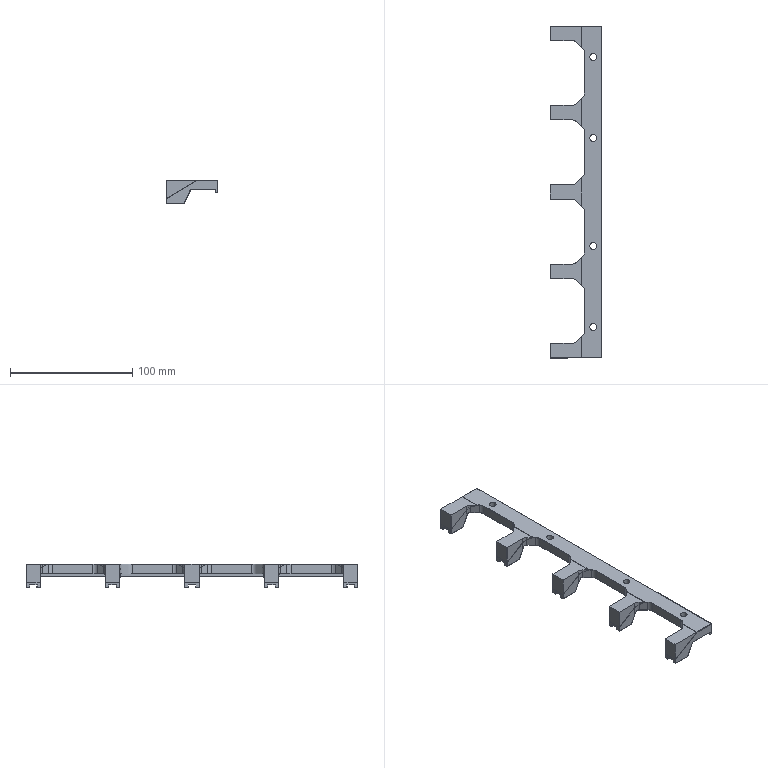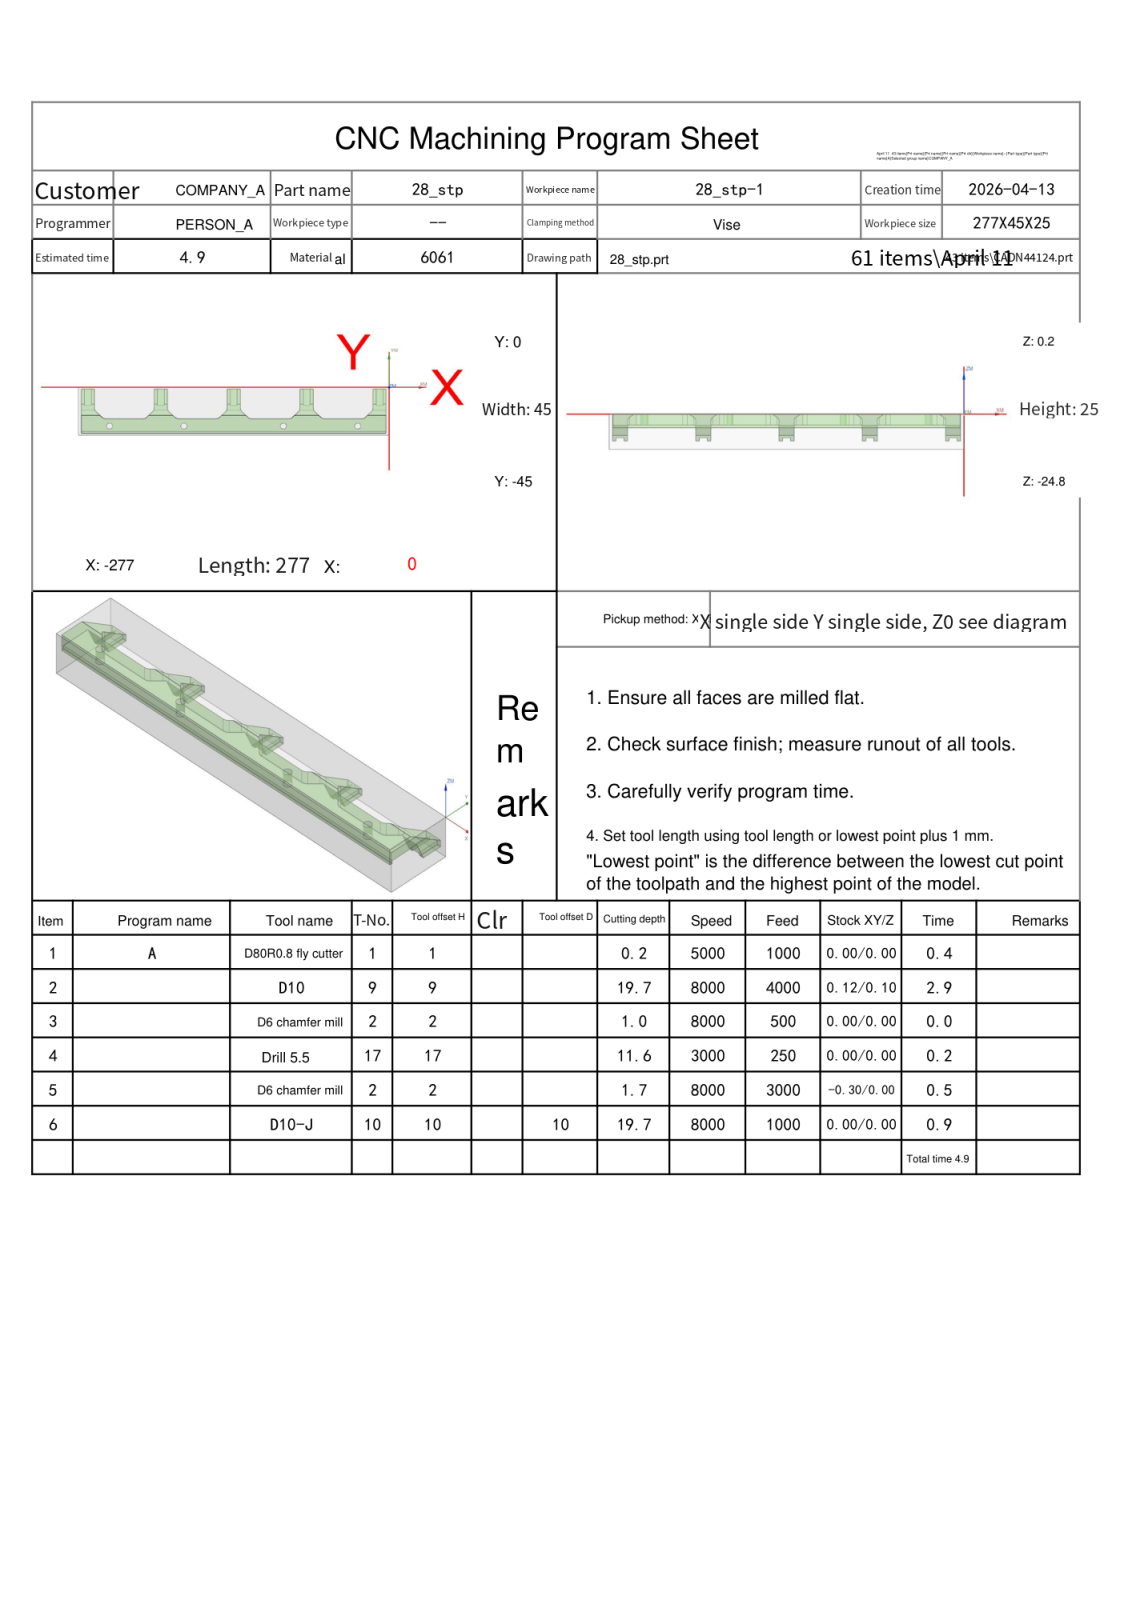NC program | NX | posted by the shop | part box 42 x 271.8 x 19 mm
Lines 2488 to 2830 of 2830:
N3 T02 M06
(D6 chamfer mill  D=6. R=0. H=02 ce=0.00 di=0.10)
G00 G90 G54 X-27.9 Y-36.5 M03 S8000
G43 H02 Z20.
M08
G98 G81 X-27.9 Y-36.5 Z-.8 R1. F500.
X-94.2
X-182.8
X-249.1
G80
G00 Z20.
G91 G28 Z0.0
M05
M09
G91 G28 Z0.0
M01
N4 T17 M06
(drill 5.5 D=5.5 DR_a=118 H=17)
G00 G90 G54 X-27.9 Y-36.5 M03 S3000
G43 H17 Z20.
M08
G98 G83 X-27.9 Y-36.5 Z-11.402 R1. F250. Q3.
X-94.2
X-182.8
X-249.1
G80
G00 Z20.
G91 G28 Z0.0
M05
M09
G91 G28 Z0.0
M01
N5 T02 M06
(D6 chamfer mill  D=6. R=0. H=02 ce=0.00 di=0.00)
G00 G90 G54 X-138.25 Y-45.628 M03 S8000
G43 H02 Z20.
M08
Z2.099
G01 Z-1.499 F3000.
G03 X-138.17 Y-45.328 I-.52 J.3
X-138.47 Y-44.808 I-.6 J0.0
G01 X-138.5 Y-44.8
X-273.9
X-274.154 Y-44.775
X-274.397 Y-44.701
X-274.622 Y-44.581
X-274.819 Y-44.419
X-275.319 Y-43.919
X-275.481 Y-43.722
X-275.601 Y-43.497
X-275.675 Y-43.254
X-275.7 Y-43.
Y-1.7
X-275.675 Y-1.446
X-275.601 Y-1.203
X-275.481 Y-.978
X-275.319 Y-.781
X-275.119 Y-.581
X-274.922 Y-.419
X-274.697 Y-.299
X-274.454 Y-.225
X-274.2 Y-.2
X-262.7
X-262.446 Y-.225
X-262.203 Y-.299
X-261.978 Y-.419
X-261.781 Y-.581
X-261.581 Y-.781
X-261.419 Y-.978
X-261.299 Y-1.203
X-261.225 Y-1.446
X-261.2 Y-1.7
Y-19.429
G03 X-260.116 Y-22.045 I3.7 J0.0
G01 X-255.045 Y-27.116
G03 X-252.429 Y-28.2 I2.616 J2.616
G01 X-219.571
G03 X-216.955 Y-27.116 I0.0 J3.7
G01 X-211.884 Y-22.045
G03 X-210.8 Y-19.429 I-2.616 J2.616
G01 Y-1.7
X-210.775 Y-1.446
X-210.701 Y-1.203
X-210.581 Y-.978
X-210.419 Y-.781
X-210.219 Y-.581
X-210.022 Y-.419
X-209.797 Y-.299
X-209.554 Y-.225
X-209.3 Y-.2
X-197.7
X-197.446 Y-.225
X-197.203 Y-.299
X-196.978 Y-.419
X-196.781 Y-.581
X-196.581 Y-.781
X-196.419 Y-.978
X-196.299 Y-1.203
X-196.225 Y-1.446
X-196.2 Y-1.7
Y-19.429
G03 X-195.116 Y-22.045 I3.7 J0.0
G01 X-190.045 Y-27.116
G03 X-187.429 Y-28.2 I2.616 J2.616
G01 X-154.571
G03 X-151.955 Y-27.116 I0.0 J3.7
G01 X-146.884 Y-22.045
G03 X-145.8 Y-19.429 I-2.616 J2.616
G01 Y-1.7
X-145.775 Y-1.446
X-145.701 Y-1.203
X-145.581 Y-.978
X-145.419 Y-.781
X-145.219 Y-.581
X-145.022 Y-.419
X-144.797 Y-.299
X-144.554 Y-.225
X-144.3 Y-.2
X-132.7
X-132.446 Y-.225
X-132.203 Y-.299
X-131.978 Y-.419
X-131.781 Y-.581
X-131.581 Y-.781
X-131.419 Y-.978
X-131.299 Y-1.203
X-131.225 Y-1.446
X-131.2 Y-1.7
Y-19.429
G03 X-130.116 Y-22.045 I3.7 J0.0
G01 X-125.045 Y-27.116
G03 X-122.429 Y-28.2 I2.616 J2.616
G01 X-89.571
G03 X-86.955 Y-27.116 I0.0 J3.7
G01 X-81.884 Y-22.045
G03 X-80.8 Y-19.429 I-2.616 J2.616
G01 Y-1.7
X-80.775 Y-1.446
X-80.701 Y-1.203
X-80.581 Y-.978
X-80.419 Y-.781
X-80.219 Y-.581
X-80.022 Y-.419
X-79.797 Y-.299
X-79.554 Y-.225
X-79.3 Y-.2
X-67.7
X-67.446 Y-.225
X-67.203 Y-.299
X-66.978 Y-.419
X-66.781 Y-.581
X-66.581 Y-.781
X-66.419 Y-.978
X-66.299 Y-1.203
X-66.225 Y-1.446
X-66.2 Y-1.7
Y-19.429
G03 X-65.116 Y-22.045 I3.7 J0.0
G01 X-60.045 Y-27.116
G03 X-57.429 Y-28.2 I2.616 J2.616
G01 X-24.571
G03 X-21.955 Y-27.116 I0.0 J3.7
G01 X-16.884 Y-22.045
G03 X-15.8 Y-19.429 I-2.616 J2.616
G01 Y-1.7
X-15.775 Y-1.446
X-15.701 Y-1.203
X-15.581 Y-.978
X-15.419 Y-.781
X-15.219 Y-.581
X-15.022 Y-.419
X-14.797 Y-.299
X-14.554 Y-.225
X-14.3 Y-.2
X-2.8
X-2.546 Y-.225
X-2.303 Y-.299
X-2.078 Y-.419
X-1.881 Y-.581
X-1.681 Y-.781
X-1.519 Y-.978
X-1.399 Y-1.203
X-1.325 Y-1.446
X-1.3 Y-1.7
Y-43.
X-1.325 Y-43.254
X-1.399 Y-43.497
X-1.519 Y-43.722
X-1.681 Y-43.919
X-2.181 Y-44.419
X-2.378 Y-44.581
X-2.603 Y-44.701
X-2.846 Y-44.775
X-3.1 Y-44.8
X-138.5
X-138.53 Y-44.808
G03 X-138.83 Y-45.328 I.3 J-.52
X-138.75 Y-45.628 I.6 J0.0
G01 Z2.099
G00 Z20.
G00 G90 X-248.114 Y-36.139 M03 S8000
Z20.
Z-.5
G01 Z-1. F500.
X-247.6 Y-35.95
G03 X-249.1 Y-34.45 I-1.5 J0.0
X-251.15 Y-36.5 I0.0 J-2.05
X-249.1 Y-38.55 I2.05 J0.0
X-247.05 Y-36.5 I0.0 J2.05
X-249.1 Y-34.45 I-2.05 J0.0
X-250.6 Y-35.95 I0.0 J-1.5
G01 X-250.086 Y-36.139
Z-.5
G00 Z20.
X-181.814
Z-.5
G01 Z-1.
X-181.3 Y-35.95
G03 X-182.8 Y-34.45 I-1.5 J0.0
X-184.85 Y-36.5 I0.0 J-2.05
X-182.8 Y-38.55 I2.05 J0.0
X-180.75 Y-36.5 I0.0 J2.05
X-182.8 Y-34.45 I-2.05 J0.0
X-184.3 Y-35.95 I0.0 J-1.5
G01 X-183.786 Y-36.139
Z-.5
G00 Z20.
X-93.214
Z-.5
G01 Z-1.
X-92.7 Y-35.95
G03 X-94.2 Y-34.45 I-1.5 J0.0
X-96.25 Y-36.5 I0.0 J-2.05
X-94.2 Y-38.55 I2.05 J0.0
X-92.15 Y-36.5 I0.0 J2.05
X-94.2 Y-34.45 I-2.05 J0.0
X-95.7 Y-35.95 I0.0 J-1.5
G01 X-95.186 Y-36.139
Z-.5
G00 Z20.
X-26.914
Z-.5
G01 Z-1.
X-26.4 Y-35.95
G03 X-27.9 Y-34.45 I-1.5 J0.0
X-29.95 Y-36.5 I0.0 J-2.05
X-27.9 Y-38.55 I2.05 J0.0
X-25.85 Y-36.5 I0.0 J2.05
X-27.9 Y-34.45 I-2.05 J0.0
X-29.4 Y-35.95 I0.0 J-1.5
G01 X-28.886 Y-36.139
Z-.5
G00 Z20.
G91 G28 Z0.0
M05
M09
G91 G28 Z0.0
M01
N6 T10 M06
(D10-J  D=10. R=0. H=10 ce=0.00 di=0.00)
G00 G90 G54 X-2.087 Y-49.616 M03 S8000
G43 H10 Z20.
M08
Z-19.
G01 Z-19.5 F1000.
G41 D10
X-2.103 Y-49.417
G03 X-3.1 Y-48.5 I-.997 J-.083
G01 X-273.9
G02 X-277.436 Y-47.036 I0.0 J5.
G01 X-277.936 Y-46.536
G02 X-279.4 Y-43. I3.536 J3.536
G01 Y-1.7
G02 X-277.936 Y1.836 I5. J0.0
G01 X-277.736 Y2.036
G02 X-274.2 Y3.5 I3.536 J-3.536
G01 X-262.7
G02 X-259.164 Y2.036 I0.0 J-5.
G01 X-258.964 Y1.836
G02 X-257.5 Y-1.7 I-3.536 J-3.536
G01 Y-19.429
X-252.429 Y-24.5
X-219.571
X-214.5 Y-19.429
Y-1.7
G02 X-213.036 Y1.836 I5. J0.0
G01 X-212.836 Y2.036
G02 X-209.3 Y3.5 I3.536 J-3.536
G01 X-197.7
G02 X-194.164 Y2.036 I0.0 J-5.
G01 X-193.964 Y1.836
G02 X-192.5 Y-1.7 I-3.536 J-3.536
G01 Y-19.429
X-187.429 Y-24.5
X-154.571
X-149.5 Y-19.429
Y-1.7
G02 X-148.036 Y1.836 I5. J0.0
G01 X-147.836 Y2.036
G02 X-144.3 Y3.5 I3.536 J-3.536
G01 X-132.7
G02 X-129.164 Y2.036 I0.0 J-5.
G01 X-128.964 Y1.836
G02 X-127.5 Y-1.7 I-3.536 J-3.536
G01 Y-19.429
X-122.429 Y-24.5
X-89.571
X-84.5 Y-19.429
Y-1.7
G02 X-83.036 Y1.836 I5. J0.0
G01 X-82.836 Y2.036
G02 X-79.3 Y3.5 I3.536 J-3.536
G01 X-67.7
G02 X-64.164 Y2.036 I0.0 J-5.
G01 X-63.964 Y1.836
G02 X-62.5 Y-1.7 I-3.536 J-3.536
G01 Y-19.429
X-57.429 Y-24.5
X-24.571
X-19.5 Y-19.429
Y-1.7
G02 X-18.036 Y1.836 I5. J0.0
G01 X-17.836 Y2.036
G02 X-14.3 Y3.5 I3.536 J-3.536
G01 X-2.8
G02 X.736 Y2.036 I0.0 J-5.
G01 X.936 Y1.836
G02 X2.4 Y-1.7 I-3.536 J-3.536
G01 Y-43.
G02 X.936 Y-46.536 I-5. J0.0
G01 X.436 Y-47.036
G02 X-3.1 Y-48.5 I-3.536 J3.536
G01 X-3.6
G03 X-4.6 Y-49.5 I0.0 J-1.
G01 G40 Y-49.7
Z-19.
G00 Z20.
M05
M09
G91 G28 Z0.0
G91 G28 Y0.0
M30
%